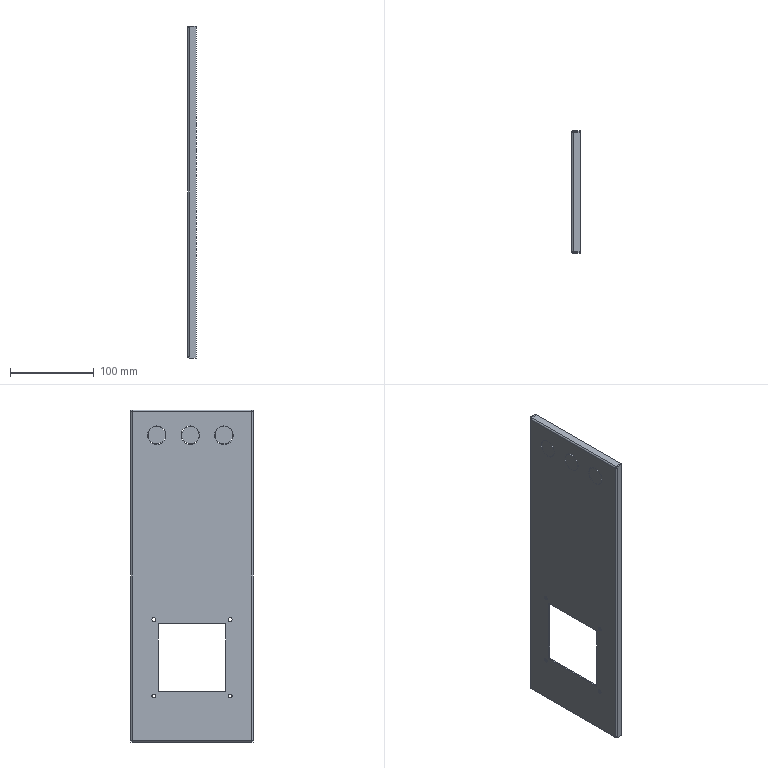Part | SolidWorks | features BaseBody 1 | 1 solid | 74 faces | box 10 x 146 x 396 mm | volume 89676 mm3 | plane 46 | cylinder 28 | commonest cylinder face diameters 4.5 x8 21 x6 22 x6 0.4 x4 3.4 x4